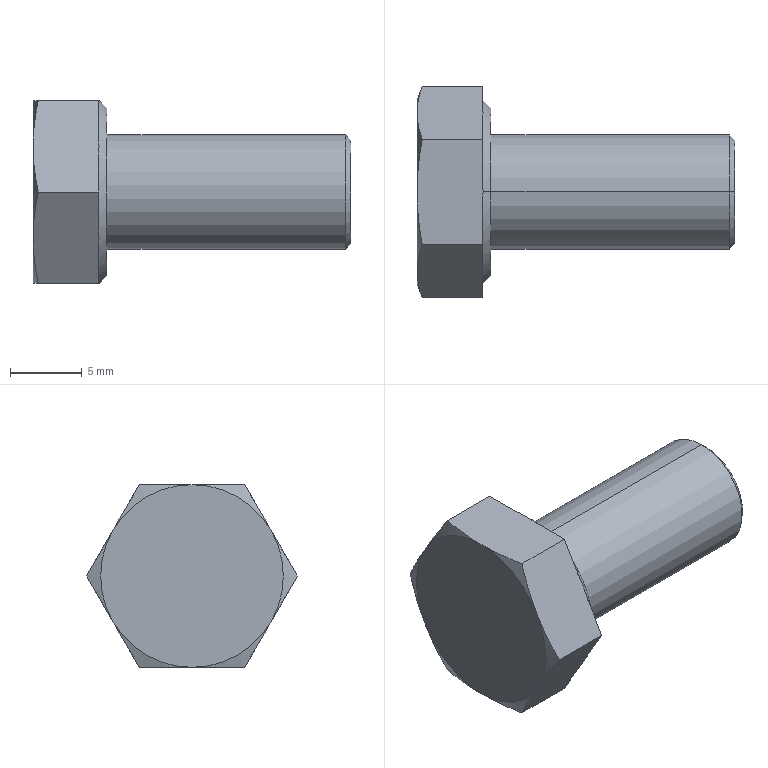Part | STEP file | hex head bolts-fine pitch grade ab gb2_GB_FASTENER_BOLT_HHBFPT A M8X1X40-N | 1 solid | 27 faces | box 22.15 x 14.699 x 12.73 mm | volume 1560 mm3 | plane 15 | cone 10 | cylinder 2 | commonest cylinder face diameters 8 x2